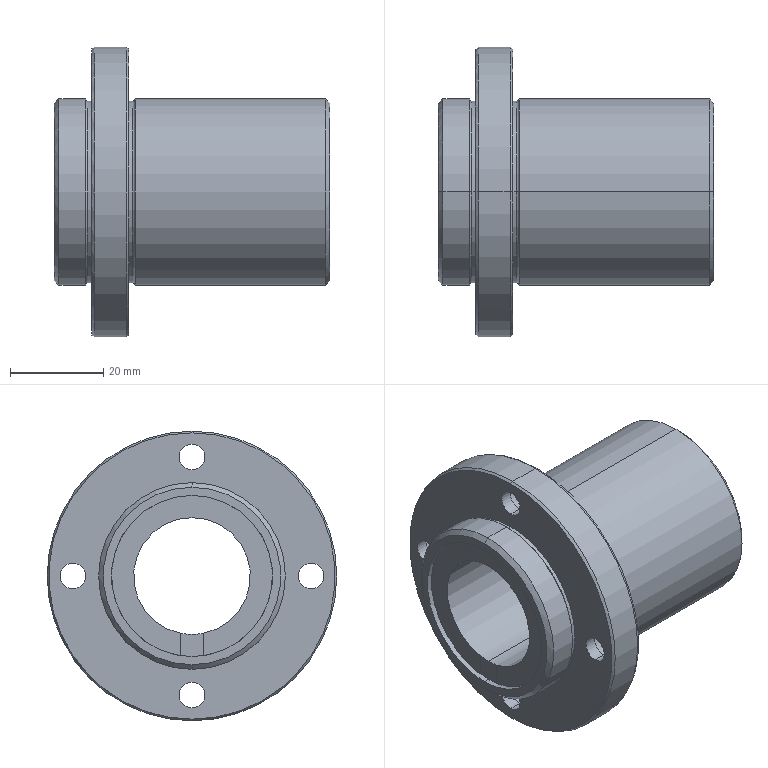Part | STEP file | 1 solid | 60 faces | box 59 x 62 x 62 mm | volume 56273 mm3 | cylinder 32 | plane 16 | cone 8 | torus 4 | commonest cylinder face diameters 5.5 x8 9 x8 34.5 x4 38.86 x4 40 x4 25 x2